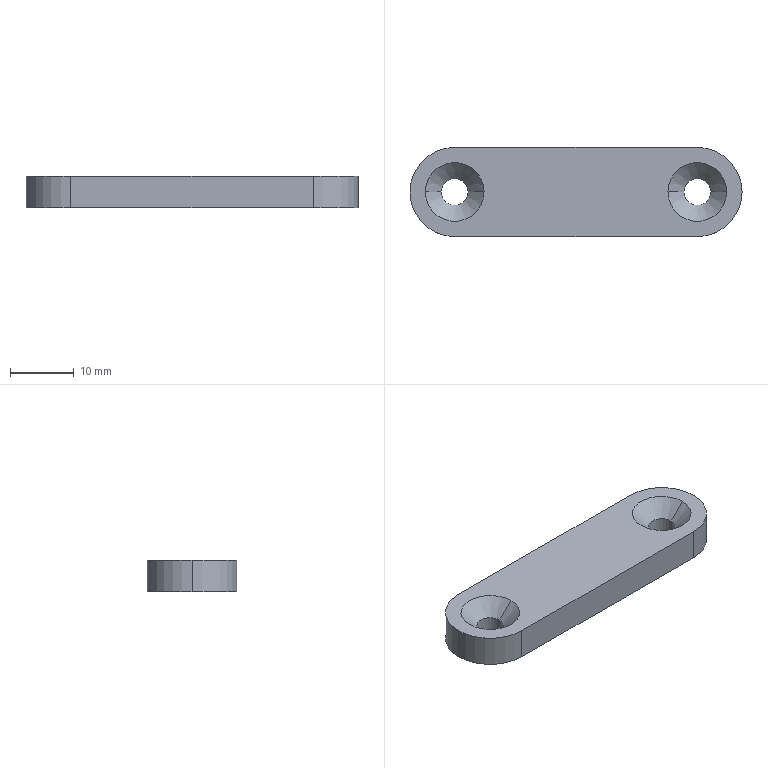Part | STEP file | Ngam kep 4 | 1 solid | 16 faces | box 52 x 14 x 5 mm | volume 3176 mm3 | cylinder 8 | cone 4 | plane 4 | commonest cylinder face diameters 4.2 x4 14 x4
STEP:
#1=CARTESIAN_POINT('',(0.,0.,0.));
#2=DIRECTION('',(0.,0.,1.));
#3=DIRECTION('',(1.,0.,0.));
#4=AXIS2_PLACEMENT_3D('',#1,#2,#3);
#5=CARTESIAN_POINT('',(-16.9,0.,2.5));
#6=VERTEX_POINT('',#5);
#7=CARTESIAN_POINT('',(-14.4,0.,5.));
#8=VERTEX_POINT('',#7);
#9=CARTESIAN_POINT('',(-16.9,0.,2.5));
#10=DIRECTION('',(0.7071,0.,0.7071));
#11=VECTOR('',#10,1.);
#12=LINE('',#9,#11);
#13=CARTESIAN_POINT('',(-19.,0.,2.5));
#14=DIRECTION('',(0.,0.,1.));
#15=DIRECTION('',(1.,0.,0.));
#16=AXIS2_PLACEMENT_3D('',#13,#14,#15);
#17=CONICAL_SURFACE('',#16,2.1,0.7854);
#18=CARTESIAN_POINT('',(6.283,0.));
#19=DIRECTION('',(0.,1.));
#20=VECTOR('',#19,1.);
#21=LINE('',#18,#20);
#22=(GEOMETRIC_REPRESENTATION_CONTEXT(2)PARAMETRIC_REPRESENTATION_CONTEXT()REPRESENTATION_CONTEXT('',''));
#23=DEFINITIONAL_REPRESENTATION('',(#21),#22);
#24=PCURVE('',#17,#23);
#25=CARTESIAN_POINT('',(-19.,0.,2.5));
#26=DIRECTION('',(0.,0.,1.));
#27=DIRECTION('',(1.,0.,0.));
#28=AXIS2_PLACEMENT_3D('',#25,#26,#27);
#29=CONICAL_SURFACE('',#28,2.1,0.7854);
#30=CARTESIAN_POINT('',(0.,0.));
#31=DIRECTION('',(0.,1.));
#32=VECTOR('',#31,1.);
#33=LINE('',#30,#32);
#34=(GEOMETRIC_REPRESENTATION_CONTEXT(2)PARAMETRIC_REPRESENTATION_CONTEXT()REPRESENTATION_CONTEXT('',''));
#35=DEFINITIONAL_REPRESENTATION('',(#33),#34);
#36=PCURVE('',#29,#35);
#37=SURFACE_CURVE('',#12,(#24,#36),.PCURVE_S1.);
#38=EDGE_CURVE('',#6,#8,#37,.T.);
#39=ORIENTED_EDGE('',*,*,#38,.T.);
#40=CARTESIAN_POINT('',(-23.6,0.,5.));
#41=VERTEX_POINT('',#40);
#42=CARTESIAN_POINT('',(-19.,0.,5.));
#43=DIRECTION('',(0.,0.,-1.));
#44=DIRECTION('',(-1.,0.,0.));
#45=AXIS2_PLACEMENT_3D('',#42,#43,#44);
#46=CIRCLE('',#45,4.6);
#47=CARTESIAN_POINT('',(9.425,2.5));
#48=DIRECTION('',(-1.,0.));
#49=VECTOR('',#48,1.);
#50=LINE('',#47,#49);
#51=(GEOMETRIC_REPRESENTATION_CONTEXT(2)PARAMETRIC_REPRESENTATION_CONTEXT()REPRESENTATION_CONTEXT('',''));
#52=DEFINITIONAL_REPRESENTATION('',(#50),#51);
#53=PCURVE('',#17,#52);
#54=CARTESIAN_POINT('',(0.,0.,5.));
#55=DIRECTION('',(0.,0.,-1.));
#56=DIRECTION('',(-1.,0.,0.));
#57=AXIS2_PLACEMENT_3D('',#54,#55,#56);
#58=PLANE('',#57);
#59=CARTESIAN_POINT('',(19.,0.));
#60=DIRECTION('',(1.,0.));
#61=AXIS2_PLACEMENT_2D('',#59,#60);
#62=CIRCLE('',#61,4.6);
#63=(GEOMETRIC_REPRESENTATION_CONTEXT(2)PARAMETRIC_REPRESENTATION_CONTEXT()REPRESENTATION_CONTEXT('',''));
#64=DEFINITIONAL_REPRESENTATION('',(#62),#63);
#65=PCURVE('',#58,#64);
#66=SURFACE_CURVE('',#46,(#53,#65),.PCURVE_S1.);
#67=EDGE_CURVE('',#8,#41,#66,.T.);
#68=ORIENTED_EDGE('',*,*,#67,.T.);
#69=CARTESIAN_POINT('',(-21.1,0.,2.5));
#70=VERTEX_POINT('',#69);
#71=CARTESIAN_POINT('',(-21.1,0.,2.5));
#72=DIRECTION('',(-0.7071,0.,0.7071));
#73=VECTOR('',#72,1.);
#74=LINE('',#71,#73);
#75=CARTESIAN_POINT('',(3.142,0.));
#76=DIRECTION('',(0.,1.));
#77=VECTOR('',#76,1.);
#78=LINE('',#75,#77);
#79=(GEOMETRIC_REPRESENTATION_CONTEXT(2)PARAMETRIC_REPRESENTATION_CONTEXT()REPRESENTATION_CONTEXT('',''));
#80=DEFINITIONAL_REPRESENTATION('',(#78),#79);
#81=PCURVE('',#17,#80);
#82=CARTESIAN_POINT('',(3.142,0.));
#83=DIRECTION('',(0.,1.));
#84=VECTOR('',#83,1.);
#85=LINE('',#82,#84);
#86=(GEOMETRIC_REPRESENTATION_CONTEXT(2)PARAMETRIC_REPRESENTATION_CONTEXT()REPRESENTATION_CONTEXT('',''));
#87=DEFINITIONAL_REPRESENTATION('',(#85),#86);
#88=PCURVE('',#29,#87);
#89=SURFACE_CURVE('',#74,(#81,#88),.PCURVE_S1.);
#90=EDGE_CURVE('',#70,#41,#89,.T.);
#91=ORIENTED_EDGE('',*,*,#90,.F.);
#92=CARTESIAN_POINT('',(-19.,0.,2.5));
#93=DIRECTION('',(0.,0.,1.));
#94=DIRECTION('',(-1.,0.,0.));
#95=AXIS2_PLACEMENT_3D('',#92,#93,#94);
#96=CIRCLE('',#95,2.1);
#97=CARTESIAN_POINT('',(3.142,0.));
#98=DIRECTION('',(1.,0.));
#99=VECTOR('',#98,1.);
#100=LINE('',#97,#99);
#101=(GEOMETRIC_REPRESENTATION_CONTEXT(2)PARAMETRIC_REPRESENTATION_CONTEXT()REPRESENTATION_CONTEXT('',''));
#102=DEFINITIONAL_REPRESENTATION('',(#100),#101);
#103=PCURVE('',#17,#102);
#104=CARTESIAN_POINT('',(-19.,0.,5.));
#105=DIRECTION('',(0.,0.,-1.));
#106=DIRECTION('',(-1.,0.,0.));
#107=AXIS2_PLACEMENT_3D('',#104,#105,#106);
#108=CYLINDRICAL_SURFACE('',#107,2.1);
#109=CARTESIAN_POINT('',(6.283,2.5));
#110=DIRECTION('',(-1.,0.));
#111=VECTOR('',#110,1.);
#112=LINE('',#109,#111);
#113=(GEOMETRIC_REPRESENTATION_CONTEXT(2)PARAMETRIC_REPRESENTATION_CONTEXT()REPRESENTATION_CONTEXT('',''));
#114=DEFINITIONAL_REPRESENTATION('',(#112),#113);
#115=PCURVE('',#108,#114);
#116=SURFACE_CURVE('',#96,(#103,#115),.PCURVE_S1.);
#117=EDGE_CURVE('',#70,#6,#116,.T.);
#118=ORIENTED_EDGE('',*,*,#117,.T.);
#119=EDGE_LOOP('',(#39,#68,#91,#118));
#120=FACE_BOUND('',#119,.F.);
#121=ADVANCED_FACE('',(#120),#17,.F.);
#122=CARTESIAN_POINT('',(21.1,0.,2.5));
#123=VERTEX_POINT('',#122);
#124=CARTESIAN_POINT('',(23.6,0.,5.));
#125=VERTEX_POINT('',#124);
#126=CARTESIAN_POINT('',(21.1,0.,2.5));
#127=DIRECTION('',(0.7071,0.,0.7071));
#128=VECTOR('',#127,1.);
#129=LINE('',#126,#128);
#130=CARTESIAN_POINT('',(19.,0.,2.5));
#131=DIRECTION('',(0.,0.,1.));
#132=DIRECTION('',(1.,0.,0.));
#133=AXIS2_PLACEMENT_3D('',#130,#131,#132);
#134=CONICAL_SURFACE('',#133,2.1,0.7854);
#135=CARTESIAN_POINT('',(6.283,0.));
#136=DIRECTION('',(0.,1.));
#137=VECTOR('',#136,1.);
#138=LINE('',#135,#137);
#139=(GEOMETRIC_REPRESENTATION_CONTEXT(2)PARAMETRIC_REPRESENTATION_CONTEXT()REPRESENTATION_CONTEXT('',''));
#140=DEFINITIONAL_REPRESENTATION('',(#138),#139);
#141=PCURVE('',#134,#140);
#142=CARTESIAN_POINT('',(19.,0.,2.5));
#143=DIRECTION('',(0.,0.,1.));
#144=DIRECTION('',(1.,0.,0.));
#145=AXIS2_PLACEMENT_3D('',#142,#143,#144);
#146=CONICAL_SURFACE('',#145,2.1,0.7854);
#147=CARTESIAN_POINT('',(0.,0.));
#148=DIRECTION('',(0.,1.));
#149=VECTOR('',#148,1.);
#150=LINE('',#147,#149);
#151=(GEOMETRIC_REPRESENTATION_CONTEXT(2)PARAMETRIC_REPRESENTATION_CONTEXT()REPRESENTATION_CONTEXT('',''));
#152=DEFINITIONAL_REPRESENTATION('',(#150),#151);
#153=PCURVE('',#146,#152);
#154=SURFACE_CURVE('',#129,(#141,#153),.PCURVE_S1.);
#155=EDGE_CURVE('',#123,#125,#154,.T.);
#156=ORIENTED_EDGE('',*,*,#155,.T.);
#157=CARTESIAN_POINT('',(14.4,0.,5.));
#158=VERTEX_POINT('',#157);
#159=CARTESIAN_POINT('',(19.,0.,5.));
#160=DIRECTION('',(0.,0.,-1.));
#161=DIRECTION('',(-1.,0.,0.));
#162=AXIS2_PLACEMENT_3D('',#159,#160,#161);
#163=CIRCLE('',#162,4.6);
#164=CARTESIAN_POINT('',(9.425,2.5));
#165=DIRECTION('',(-1.,0.));
#166=VECTOR('',#165,1.);
#167=LINE('',#164,#166);
#168=(GEOMETRIC_REPRESENTATION_CONTEXT(2)PARAMETRIC_REPRESENTATION_CONTEXT()REPRESENTATION_CONTEXT('',''));
#169=DEFINITIONAL_REPRESENTATION('',(#167),#168);
#170=PCURVE('',#134,#169);
#171=CARTESIAN_POINT('',(-19.,0.));
#172=DIRECTION('',(1.,0.));
#173=AXIS2_PLACEMENT_2D('',#171,#172);
#174=CIRCLE('',#173,4.6);
#175=(GEOMETRIC_REPRESENTATION_CONTEXT(2)PARAMETRIC_REPRESENTATION_CONTEXT()REPRESENTATION_CONTEXT('',''));
#176=DEFINITIONAL_REPRESENTATION('',(#174),#175);
#177=PCURVE('',#58,#176);
#178=SURFACE_CURVE('',#163,(#170,#177),.PCURVE_S1.);
#179=EDGE_CURVE('',#125,#158,#178,.T.);
#180=ORIENTED_EDGE('',*,*,#179,.T.);
#181=CARTESIAN_POINT('',(16.9,0.,2.5));
#182=VERTEX_POINT('',#181);
#183=CARTESIAN_POINT('',(16.9,0.,2.5));
#184=DIRECTION('',(-0.7071,0.,0.7071));
#185=VECTOR('',#184,1.);
#186=LINE('',#183,#185);
#187=CARTESIAN_POINT('',(3.142,0.));
#188=DIRECTION('',(0.,1.));
#189=VECTOR('',#188,1.);
#190=LINE('',#187,#189);
#191=(GEOMETRIC_REPRESENTATION_CONTEXT(2)PARAMETRIC_REPRESENTATION_CONTEXT()REPRESENTATION_CONTEXT('',''));
#192=DEFINITIONAL_REPRESENTATION('',(#190),#191);
#193=PCURVE('',#134,#192);
#194=CARTESIAN_POINT('',(3.142,0.));
#195=DIRECTION('',(0.,1.));
#196=VECTOR('',#195,1.);
#197=LINE('',#194,#196);
#198=(GEOMETRIC_REPRESENTATION_CONTEXT(2)PARAMETRIC_REPRESENTATION_CONTEXT()REPRESENTATION_CONTEXT('',''));
#199=DEFINITIONAL_REPRESENTATION('',(#197),#198);
#200=PCURVE('',#146,#199);
#201=SURFACE_CURVE('',#186,(#193,#200),.PCURVE_S1.);
#202=EDGE_CURVE('',#182,#158,#201,.T.);
#203=ORIENTED_EDGE('',*,*,#202,.F.);
#204=CARTESIAN_POINT('',(19.,0.,2.5));
#205=DIRECTION('',(0.,0.,1.));
#206=DIRECTION('',(-1.,0.,0.));
#207=AXIS2_PLACEMENT_3D('',#204,#205,#206);
#208=CIRCLE('',#207,2.1);
#209=CARTESIAN_POINT('',(3.142,0.));
#210=DIRECTION('',(1.,0.));
#211=VECTOR('',#210,1.);
#212=LINE('',#209,#211);
#213=(GEOMETRIC_REPRESENTATION_CONTEXT(2)PARAMETRIC_REPRESENTATION_CONTEXT()REPRESENTATION_CONTEXT('',''));
#214=DEFINITIONAL_REPRESENTATION('',(#212),#213);
#215=PCURVE('',#134,#214);
#216=CARTESIAN_POINT('',(19.,0.,5.));
#217=DIRECTION('',(0.,0.,-1.));
#218=DIRECTION('',(-1.,0.,0.));
#219=AXIS2_PLACEMENT_3D('',#216,#217,#218);
#220=CYLINDRICAL_SURFACE('',#219,2.1);
#221=CARTESIAN_POINT('',(6.283,2.5));
#222=DIRECTION('',(-1.,0.));
#223=VECTOR('',#222,1.);
#224=LINE('',#221,#223);
#225=(GEOMETRIC_REPRESENTATION_CONTEXT(2)PARAMETRIC_REPRESENTATION_CONTEXT()REPRESENTATION_CONTEXT('',''));
#226=DEFINITIONAL_REPRESENTATION('',(#224),#225);
#227=PCURVE('',#220,#226);
#228=SURFACE_CURVE('',#208,(#215,#227),.PCURVE_S1.);
#229=EDGE_CURVE('',#182,#123,#228,.T.);
#230=ORIENTED_EDGE('',*,*,#229,.T.);
#231=EDGE_LOOP('',(#156,#180,#203,#230));
#232=FACE_BOUND('',#231,.F.);
#233=ADVANCED_FACE('',(#232),#134,.F.);
#234=CARTESIAN_POINT('',(16.9,0.,0.));
#235=VERTEX_POINT('',#234);
#236=CARTESIAN_POINT('',(16.9,0.,5.));
#237=DIRECTION('',(0.,0.,-1.));
#238=VECTOR('',#237,1.);
#239=LINE('',#236,#238);
#240=CARTESIAN_POINT('',(6.283,0.));
#241=DIRECTION('',(0.,1.));
#242=VECTOR('',#241,1.);
#243=LINE('',#240,#242);
#244=(GEOMETRIC_REPRESENTATION_CONTEXT(2)PARAMETRIC_REPRESENTATION_CONTEXT()REPRESENTATION_CONTEXT('',''));
#245=DEFINITIONAL_REPRESENTATION('',(#243),#244);
#246=PCURVE('',#220,#245);
#247=CARTESIAN_POINT('',(19.,0.,5.));
#248=DIRECTION('',(0.,0.,-1.));
#249=DIRECTION('',(-1.,0.,0.));
#250=AXIS2_PLACEMENT_3D('',#247,#248,#249);
#251=CYLINDRICAL_SURFACE('',#250,2.1);
#252=CARTESIAN_POINT('',(0.,0.));
#253=DIRECTION('',(0.,1.));
#254=VECTOR('',#253,1.);
#255=LINE('',#252,#254);
#256=(GEOMETRIC_REPRESENTATION_CONTEXT(2)PARAMETRIC_REPRESENTATION_CONTEXT()REPRESENTATION_CONTEXT('',''));
#257=DEFINITIONAL_REPRESENTATION('',(#255),#256);
#258=PCURVE('',#251,#257);
#259=SURFACE_CURVE('',#239,(#246,#258),.PCURVE_S1.);
#260=EDGE_CURVE('',#182,#235,#259,.T.);
#261=ORIENTED_EDGE('',*,*,#260,.T.);
#262=CARTESIAN_POINT('',(21.1,0.,0.));
#263=VERTEX_POINT('',#262);
#264=CARTESIAN_POINT('',(19.,0.,0.));
#265=DIRECTION('',(0.,0.,1.));
#266=DIRECTION('',(1.,0.,0.));
#267=AXIS2_PLACEMENT_3D('',#264,#265,#266);
#268=CIRCLE('',#267,2.1);
#269=CARTESIAN_POINT('',(9.425,5.));
#270=DIRECTION('',(-1.,0.));
#271=VECTOR('',#270,1.);
#272=LINE('',#269,#271);
#273=(GEOMETRIC_REPRESENTATION_CONTEXT(2)PARAMETRIC_REPRESENTATION_CONTEXT()REPRESENTATION_CONTEXT('',''));
#274=DEFINITIONAL_REPRESENTATION('',(#272),#273);
#275=PCURVE('',#220,#274);
#276=CARTESIAN_POINT('',(0.,0.,0.));
#277=DIRECTION('',(0.,0.,-1.));
#278=DIRECTION('',(-1.,0.,0.));
#279=AXIS2_PLACEMENT_3D('',#276,#277,#278);
#280=PLANE('',#279);
#281=CARTESIAN_POINT('',(-21.1,0.));
#282=CARTESIAN_POINT('',(-21.1,3.637));
#283=CARTESIAN_POINT('',(-17.95,1.819));
#284=CARTESIAN_POINT('',(-14.8,0.));
#285=CARTESIAN_POINT('',(-17.95,-1.819));
#286=CARTESIAN_POINT('',(-21.1,-3.637));
#287=CARTESIAN_POINT('',(-21.1,0.));
#288=(BOUNDED_CURVE()B_SPLINE_CURVE(2,(#281,#282,#283,#284,#285,#286,#287),.UNSPECIFIED.,.T.,.F.)B_SPLINE_CURVE_WITH_KNOTS((1,2,2,2,2,1),(-2.094,0.,2.094,4.189,6.283,8.378),.UNSPECIFIED.)CURVE()GEOMETRIC_REPRESENTATION_ITEM()RATIONAL_B_SPLINE_CURVE((1.,0.5,1.,0.5,1.,0.5,1.))REPRESENTATION_ITEM(''));
#289=(GEOMETRIC_REPRESENTATION_CONTEXT(2)PARAMETRIC_REPRESENTATION_CONTEXT()REPRESENTATION_CONTEXT('',''));
#290=DEFINITIONAL_REPRESENTATION('',(#288),#289);
#291=PCURVE('',#280,#290);
#292=SURFACE_CURVE('',#268,(#275,#291),.PCURVE_S1.);
#293=EDGE_CURVE('',#235,#263,#292,.T.);
#294=ORIENTED_EDGE('',*,*,#293,.T.);
#295=CARTESIAN_POINT('',(21.1,0.,5.));
#296=DIRECTION('',(0.,0.,-1.));
#297=VECTOR('',#296,1.);
#298=LINE('',#295,#297);
#299=CARTESIAN_POINT('',(3.142,0.));
#300=DIRECTION('',(0.,1.));
#301=VECTOR('',#300,1.);
#302=LINE('',#299,#301);
#303=(GEOMETRIC_REPRESENTATION_CONTEXT(2)PARAMETRIC_REPRESENTATION_CONTEXT()REPRESENTATION_CONTEXT('',''));
#304=DEFINITIONAL_REPRESENTATION('',(#302),#303);
#305=PCURVE('',#220,#304);
#306=CARTESIAN_POINT('',(3.142,0.));
#307=DIRECTION('',(0.,1.));
#308=VECTOR('',#307,1.);
#309=LINE('',#306,#308);
#310=(GEOMETRIC_REPRESENTATION_CONTEXT(2)PARAMETRIC_REPRESENTATION_CONTEXT()REPRESENTATION_CONTEXT('',''));
#311=DEFINITIONAL_REPRESENTATION('',(#309),#310);
#312=PCURVE('',#251,#311);
#313=SURFACE_CURVE('',#298,(#305,#312),.PCURVE_S1.);
#314=EDGE_CURVE('',#123,#263,#313,.T.);
#315=ORIENTED_EDGE('',*,*,#314,.F.);
#316=ORIENTED_EDGE('',*,*,#229,.F.);
#317=EDGE_LOOP('',(#261,#294,#315,#316));
#318=FACE_BOUND('',#317,.F.);
#319=ADVANCED_FACE('',(#318),#220,.F.);
#320=CARTESIAN_POINT('',(-21.1,0.,0.));
#321=VERTEX_POINT('',#320);
#322=CARTESIAN_POINT('',(-21.1,0.,5.));
#323=DIRECTION('',(0.,0.,-1.));
#324=VECTOR('',#323,1.);
#325=LINE('',#322,#324);
#326=CARTESIAN_POINT('',(6.283,0.));
#327=DIRECTION('',(0.,1.));
#328=VECTOR('',#327,1.);
#329=LINE('',#326,#328);
#330=(GEOMETRIC_REPRESENTATION_CONTEXT(2)PARAMETRIC_REPRESENTATION_CONTEXT()REPRESENTATION_CONTEXT('',''));
#331=DEFINITIONAL_REPRESENTATION('',(#329),#330);
#332=PCURVE('',#108,#331);
#333=CARTESIAN_POINT('',(-19.,0.,5.));
#334=DIRECTION('',(0.,0.,-1.));
#335=DIRECTION('',(-1.,0.,0.));
#336=AXIS2_PLACEMENT_3D('',#333,#334,#335);
#337=CYLINDRICAL_SURFACE('',#336,2.1);
#338=CARTESIAN_POINT('',(0.,0.));
#339=DIRECTION('',(0.,1.));
#340=VECTOR('',#339,1.);
#341=LINE('',#338,#340);
#342=(GEOMETRIC_REPRESENTATION_CONTEXT(2)PARAMETRIC_REPRESENTATION_CONTEXT()REPRESENTATION_CONTEXT('',''));
#343=DEFINITIONAL_REPRESENTATION('',(#341),#342);
#344=PCURVE('',#337,#343);
#345=SURFACE_CURVE('',#325,(#332,#344),.PCURVE_S1.);
#346=EDGE_CURVE('',#70,#321,#345,.T.);
#347=ORIENTED_EDGE('',*,*,#346,.T.);
#348=CARTESIAN_POINT('',(-16.9,0.,0.));
#349=VERTEX_POINT('',#348);
#350=CARTESIAN_POINT('',(-19.,0.,0.));
#351=DIRECTION('',(0.,0.,1.));
#352=DIRECTION('',(1.,0.,0.));
#353=AXIS2_PLACEMENT_3D('',#350,#351,#352);
#354=CIRCLE('',#353,2.1);
#355=CARTESIAN_POINT('',(9.425,5.));
#356=DIRECTION('',(-1.,0.));
#357=VECTOR('',#356,1.);
#358=LINE('',#355,#357);
#359=(GEOMETRIC_REPRESENTATION_CONTEXT(2)PARAMETRIC_REPRESENTATION_CONTEXT()REPRESENTATION_CONTEXT('',''));
#360=DEFINITIONAL_REPRESENTATION('',(#358),#359);
#361=PCURVE('',#108,#360);
#362=CARTESIAN_POINT('',(16.9,0.));
#363=CARTESIAN_POINT('',(16.9,3.637));
#364=CARTESIAN_POINT('',(20.05,1.819));
#365=CARTESIAN_POINT('',(23.2,0.));
#366=CARTESIAN_POINT('',(20.05,-1.819));
#367=CARTESIAN_POINT('',(16.9,-3.637));
#368=CARTESIAN_POINT('',(16.9,0.));
#369=(BOUNDED_CURVE()B_SPLINE_CURVE(2,(#362,#363,#364,#365,#366,#367,#368),.UNSPECIFIED.,.T.,.F.)B_SPLINE_CURVE_WITH_KNOTS((1,2,2,2,2,1),(-2.094,0.,2.094,4.189,6.283,8.378),.UNSPECIFIED.)CURVE()GEOMETRIC_REPRESENTATION_ITEM()RATIONAL_B_SPLINE_CURVE((1.,0.5,1.,0.5,1.,0.5,1.))REPRESENTATION_ITEM(''));
#370=(GEOMETRIC_REPRESENTATION_CONTEXT(2)PARAMETRIC_REPRESENTATION_CONTEXT()REPRESENTATION_CONTEXT('',''));
#371=DEFINITIONAL_REPRESENTATION('',(#369),#370);
#372=PCURVE('',#280,#371);
#373=SURFACE_CURVE('',#354,(#361,#372),.PCURVE_S1.);
#374=EDGE_CURVE('',#321,#349,#373,.T.);
#375=ORIENTED_EDGE('',*,*,#374,.T.);
#376=CARTESIAN_POINT('',(-16.9,0.,5.));
#377=DIRECTION('',(0.,0.,-1.));
#378=VECTOR('',#377,1.);
#379=LINE('',#376,#378);
#380=CARTESIAN_POINT('',(3.142,0.));
#381=DIRECTION('',(0.,1.));
#382=VECTOR('',#381,1.);
#383=LINE('',#380,#382);
#384=(GEOMETRIC_REPRESENTATION_CONTEXT(2)PARAMETRIC_REPRESENTATION_CONTEXT()REPRESENTATION_CONTEXT('',''));
#385=DEFINITIONAL_REPRESENTATION('',(#383),#384);
#386=PCURVE('',#108,#385);
#387=CARTESIAN_POINT('',(3.142,0.));
#388=DIRECTION('',(0.,1.));
#389=VECTOR('',#388,1.);
#390=LINE('',#387,#389);
#391=(GEOMETRIC_REPRESENTATION_CONTEXT(2)PARAMETRIC_REPRESENTATION_CONTEXT()REPRESENTATION_CONTEXT('',''));
#392=DEFINITIONAL_REPRESENTATION('',(#390),#391);
#393=PCURVE('',#337,#392);
#394=SURFACE_CURVE('',#379,(#386,#393),.PCURVE_S1.);
#395=EDGE_CURVE('',#6,#349,#394,.T.);
#396=ORIENTED_EDGE('',*,*,#395,.F.);
#397=ORIENTED_EDGE('',*,*,#117,.F.);
#398=EDGE_LOOP('',(#347,#375,#396,#397));
#399=FACE_BOUND('',#398,.F.);
#400=ADVANCED_FACE('',(#399),#108,.F.);
#401=ORIENTED_EDGE('',*,*,#179,.T.);
#402=CARTESIAN_POINT('',(19.,0.,5.));
#403=DIRECTION('',(0.,0.,-1.));
#404=DIRECTION('',(-1.,0.,0.));
#405=AXIS2_PLACEMENT_3D('',#402,#403,#404);
#406=CIRCLE('',#405,4.6);
#407=CARTESIAN_POINT('',(-19.,0.));
#408=DIRECTION('',(1.,0.));
#409=AXIS2_PLACEMENT_2D('',#407,#408);
#410=CIRCLE('',#409,4.6);
#411=(GEOMETRIC_REPRESENTATION_CONTEXT(2)PARAMETRIC_REPRESENTATION_CONTEXT()REPRESENTATION_CONTEXT('',''));
#412=DEFINITIONAL_REPRESENTATION('',(#410),#411);
#413=PCURVE('',#58,#412);
#414=CARTESIAN_POINT('',(3.142,2.5));
#415=DIRECTION('',(-1.,0.));
#416=VECTOR('',#415,1.);
#417=LINE('',#414,#416);
#418=(GEOMETRIC_REPRESENTATION_CONTEXT(2)PARAMETRIC_REPRESENTATION_CONTEXT()REPRESENTATION_CONTEXT('',''));
#419=DEFINITIONAL_REPRESENTATION('',(#417),#418);
#420=PCURVE('',#146,#419);
#421=SURFACE_CURVE('',#406,(#413,#420),.PCURVE_S1.);
#422=EDGE_CURVE('',#158,#125,#421,.T.);
#423=ORIENTED_EDGE('',*,*,#422,.T.);
#424=EDGE_LOOP('',(#401,#423));
#425=FACE_BOUND('',#424,.T.);
#426=ORIENTED_EDGE('',*,*,#67,.T.);
#427=CARTESIAN_POINT('',(-19.,0.,5.));
#428=DIRECTION('',(0.,0.,-1.));
#429=DIRECTION('',(-1.,0.,0.));
#430=AXIS2_PLACEMENT_3D('',#427,#428,#429);
#431=CIRCLE('',#430,4.6);
#432=CARTESIAN_POINT('',(19.,0.));
#433=DIRECTION('',(1.,0.));
#434=AXIS2_PLACEMENT_2D('',#432,#433);
#435=CIRCLE('',#434,4.6);
#436=(GEOMETRIC_REPRESENTATION_CONTEXT(2)PARAMETRIC_REPRESENTATION_CONTEXT()REPRESENTATION_CONTEXT('',''));
#437=DEFINITIONAL_REPRESENTATION('',(#435),#436);
#438=PCURVE('',#58,#437);
#439=CARTESIAN_POINT('',(3.142,2.5));
#440=DIRECTION('',(-1.,0.));
#441=VECTOR('',#440,1.);
#442=LINE('',#439,#441);
#443=(GEOMETRIC_REPRESENTATION_CONTEXT(2)PARAMETRIC_REPRESENTATION_CONTEXT()REPRESENTATION_CONTEXT('',''));
#444=DEFINITIONAL_REPRESENTATION('',(#442),#443);
#445=PCURVE('',#29,#444);
#446=SURFACE_CURVE('',#431,(#438,#445),.PCURVE_S1.);
#447=EDGE_CURVE('',#41,#8,#446,.T.);
#448=ORIENTED_EDGE('',*,*,#447,.T.);
#449=EDGE_LOOP('',(#426,#448));
#450=FACE_BOUND('',#449,.T.);
#451=CARTESIAN_POINT('',(-19.,7.,5.));
#452=VERTEX_POINT('',#451);
#453=CARTESIAN_POINT('',(-26.,0.,5.));
#454=VERTEX_POINT('',#453);
#455=CARTESIAN_POINT('',(-19.,0.,5.));
#456=DIRECTION('',(0.,0.,1.));
#457=DIRECTION('',(-1.,0.,0.));
#458=AXIS2_PLACEMENT_3D('',#455,#456,#457);
#459=CIRCLE('',#458,7.);
#460=CARTESIAN_POINT('',(26.,0.));
#461=CARTESIAN_POINT('',(26.,-12.124));
#462=CARTESIAN_POINT('',(15.5,-6.062));
#463=CARTESIAN_POINT('',(5.,0.));
#464=CARTESIAN_POINT('',(15.5,6.062));
#465=CARTESIAN_POINT('',(26.,12.124));
#466=CARTESIAN_POINT('',(26.,0.));
#467=(BOUNDED_CURVE()B_SPLINE_CURVE(2,(#460,#461,#462,#463,#464,#465,#466),.UNSPECIFIED.,.T.,.F.)B_SPLINE_CURVE_WITH_KNOTS((1,2,2,2,2,1),(-2.094,0.,2.094,4.189,6.283,8.378),.UNSPECIFIED.)CURVE()GEOMETRIC_REPRESENTATION_ITEM()RATIONAL_B_SPLINE_CURVE((1.,0.5,1.,0.5,1.,0.5,1.))REPRESENTATION_ITEM(''));
#468=(GEOMETRIC_REPRESENTATION_CONTEXT(2)PARAMETRIC_REPRESENTATION_CONTEXT()REPRESENTATION_CONTEXT('',''));
#469=DEFINITIONAL_REPRESENTATION('',(#467),#468);
#470=PCURVE('',#58,#469);
#471=CARTESIAN_POINT('',(-19.,0.,5.));
#472=DIRECTION('',(0.,0.,-1.));
#473=DIRECTION('',(-1.,0.,0.));
#474=AXIS2_PLACEMENT_3D('',#471,#472,#473);
#475=CYLINDRICAL_SURFACE('',#474,7.);
#476=CARTESIAN_POINT('',(6.283,0.));
#477=DIRECTION('',(-1.,0.));
#478=VECTOR('',#477,1.);
#479=LINE('',#476,#478);
#480=(GEOMETRIC_REPRESENTATION_CONTEXT(2)PARAMETRIC_REPRESENTATION_CONTEXT()REPRESENTATION_CONTEXT('',''));
#481=DEFINITIONAL_REPRESENTATION('',(#479),#480);
#482=PCURVE('',#475,#481);
#483=SURFACE_CURVE('',#459,(#470,#482),.PCURVE_S1.);
#484=EDGE_CURVE('',#452,#454,#483,.T.);
#485=ORIENTED_EDGE('',*,*,#484,.T.);
#486=CARTESIAN_POINT('',(-19.,-7.,5.));
#487=VERTEX_POINT('',#486);
#488=CARTESIAN_POINT('',(-19.,0.,5.));
#489=DIRECTION('',(0.,0.,1.));
#490=DIRECTION('',(-1.,0.,0.));
#491=AXIS2_PLACEMENT_3D('',#488,#489,#490);
#492=CIRCLE('',#491,7.);
#493=CARTESIAN_POINT('',(26.,0.));
#494=CARTESIAN_POINT('',(26.,-12.124));
#495=CARTESIAN_POINT('',(15.5,-6.062));
#496=CARTESIAN_POINT('',(5.,0.));
#497=CARTESIAN_POINT('',(15.5,6.062));
#498=CARTESIAN_POINT('',(26.,12.124));
#499=CARTESIAN_POINT('',(26.,0.));
#500=(BOUNDED_CURVE()B_SPLINE_CURVE(2,(#493,#494,#495,#496,#497,#498,#499),.UNSPECIFIED.,.T.,.F.)B_SPLINE_CURVE_WITH_KNOTS((1,2,2,2,2,1),(-2.094,0.,2.094,4.189,6.283,8.378),.UNSPECIFIED.)CURVE()GEOMETRIC_REPRESENTATION_ITEM()RATIONAL_B_SPLINE_CURVE((1.,0.5,1.,0.5,1.,0.5,1.))REPRESENTATION_ITEM(''));
#501=(GEOMETRIC_REPRESENTATION_CONTEXT(2)PARAMETRIC_REPRESENTATION_CONTEXT()REPRESENTATION_CONTEXT('',''));
#502=DEFINITIONAL_REPRESENTATION('',(#500),#501);
#503=PCURVE('',#58,#502);
#504=CARTESIAN_POINT('',(-19.,0.,5.));
#505=DIRECTION('',(0.,0.,-1.));
#506=DIRECTION('',(-1.,0.,0.));
#507=AXIS2_PLACEMENT_3D('',#504,#505,#506);
#508=CYLINDRICAL_SURFACE('',#507,7.);
#509=CARTESIAN_POINT('',(6.283,0.));
#510=DIRECTION('',(-1.,0.));
#511=VECTOR('',#510,1.);
#512=LINE('',#509,#511);
#513=(GEOMETRIC_REPRESENTATION_CONTEXT(2)PARAMETRIC_REPRESENTATION_CONTEXT()REPRESENTATION_CONTEXT('',''));
#514=DEFINITIONAL_REPRESENTATION('',(#512),#513);
#515=PCURVE('',#508,#514);
#516=SURFACE_CURVE('',#492,(#503,#515),.PCURVE_S1.);
#517=EDGE_CURVE('',#454,#487,#516,.T.);
#518=ORIENTED_EDGE('',*,*,#517,.T.);
#519=CARTESIAN_POINT('',(19.,-7.,5.));
#520=VERTEX_POINT('',#519);
#521=CARTESIAN_POINT('',(26.,-7.,5.));
#522=DIRECTION('',(1.,0.,0.));
#523=VECTOR('',#522,1.);
#524=LINE('',#521,#523);
#525=CARTESIAN_POINT('',(-26.,-7.));
#526=DIRECTION('',(-1.,0.));
#527=VECTOR('',#526,1.);
#528=LINE('',#525,#527);
#529=(GEOMETRIC_REPRESENTATION_CONTEXT(2)PARAMETRIC_REPRESENTATION_CONTEXT()REPRESENTATION_CONTEXT('',''));
#530=DEFINITIONAL_REPRESENTATION('',(#528),#529);
#531=PCURVE('',#58,#530);
#532=CARTESIAN_POINT('',(26.,-7.,5.));
#533=DIRECTION('',(0.,1.,0.));
#534=DIRECTION('',(-1.,0.,0.));
#535=AXIS2_PLACEMENT_3D('',#532,#533,#534);
#536=PLANE('',#535);
#537=CARTESIAN_POINT('',(0.,0.));
#538=DIRECTION('',(-1.,0.));
#539=VECTOR('',#538,1.);
#540=LINE('',#537,#539);
#541=(GEOMETRIC_REPRESENTATION_CONTEXT(2)PARAMETRIC_REPRESENTATION_CONTEXT()REPRESENTATION_CONTEXT('',''));
#542=DEFINITIONAL_REPRESENTATION('',(#540),#541);
#543=PCURVE('',#536,#542);
#544=SURFACE_CURVE('',#524,(#531,#543),.PCURVE_S1.);
#545=EDGE_CURVE('',#487,#520,#544,.T.);
#546=ORIENTED_EDGE('',*,*,#545,.T.);
#547=CARTESIAN_POINT('',(26.,0.,5.));
#548=VERTEX_POINT('',#547);
#549=CARTESIAN_POINT('',(19.,0.,5.));
#550=DIRECTION('',(0.,0.,1.));
#551=DIRECTION('',(-1.,0.,0.));
#552=AXIS2_PLACEMENT_3D('',#549,#550,#551);
#553=CIRCLE('',#552,7.);
#554=CARTESIAN_POINT('',(-12.,0.));
#555=CARTESIAN_POINT('',(-12.,-12.124));
#556=CARTESIAN_POINT('',(-22.5,-6.062));
#557=CARTESIAN_POINT('',(-33.,0.));
#558=CARTESIAN_POINT('',(-22.5,6.062));
#559=CARTESIAN_POINT('',(-12.,12.124));
#560=CARTESIAN_POINT('',(-12.,0.));
#561=(BOUNDED_CURVE()B_SPLINE_CURVE(2,(#554,#555,#556,#557,#558,#559,#560),.UNSPECIFIED.,.T.,.F.)B_SPLINE_CURVE_WITH_KNOTS((1,2,2,2,2,1),(-2.094,0.,2.094,4.189,6.283,8.378),.UNSPECIFIED.)CURVE()GEOMETRIC_REPRESENTATION_ITEM()RATIONAL_B_SPLINE_CURVE((1.,0.5,1.,0.5,1.,0.5,1.))REPRESENTATION_ITEM(''));
#562=(GEOMETRIC_REPRESENTATION_CONTEXT(2)PARAMETRIC_REPRESENTATION_CONTEXT()REPRESENTATION_CONTEXT('',''));
#563=DEFINITIONAL_REPRESENTATION('',(#561),#562);
#564=PCURVE('',#58,#563);
#565=CARTESIAN_POINT('',(19.,0.,5.));
#566=DIRECTION('',(0.,0.,-1.));
#567=DIRECTION('',(-1.,0.,0.));
#568=AXIS2_PLACEMENT_3D('',#565,#566,#567);
#569=CYLINDRICAL_SURFACE('',#568,7.);
#570=CARTESIAN_POINT('',(6.283,0.));
#571=DIRECTION('',(-1.,0.));
#572=VECTOR('',#571,1.);
#573=LINE('',#570,#572);
#574=(GEOMETRIC_REPRESENTATION_CONTEXT(2)PARAMETRIC_REPRESENTATION_CONTEXT()REPRESENTATION_CONTEXT('',''));
#575=DEFINITIONAL_REPRESENTATION('',(#573),#574);
#576=PCURVE('',#569,#575);
#577=SURFACE_CURVE('',#553,(#564,#576),.PCURVE_S1.);
#578=EDGE_CURVE('',#520,#548,#577,.T.);
#579=ORIENTED_EDGE('',*,*,#578,.T.);
#580=CARTESIAN_POINT('',(19.,7.,5.));
#581=VERTEX_POINT('',#580);
#582=CARTESIAN_POINT('',(19.,0.,5.));
#583=DIRECTION('',(0.,0.,1.));
#584=DIRECTION('',(-1.,0.,0.));
#585=AXIS2_PLACEMENT_3D('',#582,#583,#584);
#586=CIRCLE('',#585,7.);
#587=CARTESIAN_POINT('',(-12.,0.));
#588=CARTESIAN_POINT('',(-12.,-12.124));
#589=CARTESIAN_POINT('',(-22.5,-6.062));
#590=CARTESIAN_POINT('',(-33.,0.));
#591=CARTESIAN_POINT('',(-22.5,6.062));
#592=CARTESIAN_POINT('',(-12.,12.124));
#593=CARTESIAN_POINT('',(-12.,0.));
#594=(BOUNDED_CURVE()B_SPLINE_CURVE(2,(#587,#588,#589,#590,#591,#592,#593),.UNSPECIFIED.,.T.,.F.)B_SPLINE_CURVE_WITH_KNOTS((1,2,2,2,2,1),(-2.094,0.,2.094,4.189,6.283,8.378),.UNSPECIFIED.)CURVE()GEOMETRIC_REPRESENTATION_ITEM()RATIONAL_B_SPLINE_CURVE((1.,0.5,1.,0.5,1.,0.5,1.))REPRESENTATION_ITEM(''));
#595=(GEOMETRIC_REPRESENTATION_CONTEXT(2)PARAMETRIC_REPRESENTATION_CONTEXT()REPRESENTATION_CONTEXT('',''));
#596=DEFINITIONAL_REPRESENTATION('',(#594),#595);
#597=PCURVE('',#58,#596);
#598=CARTESIAN_POINT('',(19.,0.,5.));
#599=DIRECTION('',(0.,0.,-1.));
#600=DIRECTION('',(-1.,0.,0.));
#601=AXIS2_PLACEMENT_3D('',#598,#599,#600);
#602=CYLINDRICAL_SURFACE('',#601,7.);
#603=CARTESIAN_POINT('',(6.283,0.));
#604=DIRECTION('',(-1.,0.));
#605=VECTOR('',#604,1.);
#606=LINE('',#603,#605);
#607=(GEOMETRIC_REPRESENTATION_CONTEXT(2)PARAMETRIC_REPRESENTATION_CONTEXT()REPRESENTATION_CONTEXT('',''));
#608=DEFINITIONAL_REPRESENTATION('',(#606),#607);
#609=PCURVE('',#602,#608);
#610=SURFACE_CURVE('',#586,(#597,#609),.PCURVE_S1.);
#611=EDGE_CURVE('',#548,#581,#610,.T.);
#612=ORIENTED_EDGE('',*,*,#611,.T.);
#613=CARTESIAN_POINT('',(-26.,7.,5.));
#614=DIRECTION('',(-1.,0.,0.));
#615=VECTOR('',#614,1.);
#616=LINE('',#613,#615);
#617=CARTESIAN_POINT('',(26.,7.));
#618=DIRECTION('',(1.,0.));
#619=VECTOR('',#618,1.);
#620=LINE('',#617,#619);
#621=(GEOMETRIC_REPRESENTATION_CONTEXT(2)PARAMETRIC_REPRESENTATION_CONTEXT()REPRESENTATION_CONTEXT('',''));
#622=DEFINITIONAL_REPRESENTATION('',(#620),#621);
#623=PCURVE('',#58,#622);
#624=CARTESIAN_POINT('',(-26.,7.,5.));
#625=DIRECTION('',(0.,-1.,0.));
#626=DIRECTION('',(0.,0.,-1.));
#627=AXIS2_PLACEMENT_3D('',#624,#625,#626);
#628=PLANE('',#627);
#629=CARTESIAN_POINT('',(0.,0.));
#630=DIRECTION('',(0.,-1.));
#631=VECTOR('',#630,1.);
#632=LINE('',#629,#631);
#633=(GEOMETRIC_REPRESENTATION_CONTEXT(2)PARAMETRIC_REPRESENTATION_CONTEXT()REPRESENTATION_CONTEXT('',''));
#634=DEFINITIONAL_REPRESENTATION('',(#632),#633);
#635=PCURVE('',#628,#634);
#636=SURFACE_CURVE('',#616,(#623,#635),.PCURVE_S1.);
#637=EDGE_CURVE('',#581,#452,#636,.T.);
#638=ORIENTED_EDGE('',*,*,#637,.T.);
#639=EDGE_LOOP('',(#485,#518,#546,#579,#612,#638));
#640=FACE_BOUND('',#639,.T.);
#641=ADVANCED_FACE('',(#425,#450,#640),#58,.F.);
#642=ORIENTED_EDGE('',*,*,#374,.T.);
#643=CARTESIAN_POINT('',(-19.,0.,0.));
#644=DIRECTION('',(0.,0.,1.));
#645=DIRECTION('',(1.,0.,0.));
#646=AXIS2_PLACEMENT_3D('',#643,#644,#645);
#647=CIRCLE('',#646,2.1);
#648=CARTESIAN_POINT('',(16.9,0.));
#649=CARTESIAN_POINT('',(16.9,3.637));
#650=CARTESIAN_POINT('',(20.05,1.819));
#651=CARTESIAN_POINT('',(23.2,0.));
#652=CARTESIAN_POINT('',(20.05,-1.819));
#653=CARTESIAN_POINT('',(16.9,-3.637));
#654=CARTESIAN_POINT('',(16.9,0.));
#655=(BOUNDED_CURVE()B_SPLINE_CURVE(2,(#648,#649,#650,#651,#652,#653,#654),.UNSPECIFIED.,.T.,.F.)B_SPLINE_CURVE_WITH_KNOTS((1,2,2,2,2,1),(-2.094,0.,2.094,4.189,6.283,8.378),.UNSPECIFIED.)CURVE()GEOMETRIC_REPRESENTATION_ITEM()RATIONAL_B_SPLINE_CURVE((1.,0.5,1.,0.5,1.,0.5,1.))REPRESENTATION_ITEM(''));
#656=(GEOMETRIC_REPRESENTATION_CONTEXT(2)PARAMETRIC_REPRESENTATION_CONTEXT()REPRESENTATION_CONTEXT('',''));
#657=DEFINITIONAL_REPRESENTATION('',(#655),#656);
#658=PCURVE('',#280,#657);
#659=CARTESIAN_POINT('',(3.142,5.));
#660=DIRECTION('',(-1.,0.));
#661=VECTOR('',#660,1.);
#662=LINE('',#659,#661);
#663=(GEOMETRIC_REPRESENTATION_CONTEXT(2)PARAMETRIC_REPRESENTATION_CONTEXT()REPRESENTATION_CONTEXT('',''));
#664=DEFINITIONAL_REPRESENTATION('',(#662),#663);
#665=PCURVE('',#337,#664);
#666=SURFACE_CURVE('',#647,(#658,#665),.PCURVE_S1.);
#667=EDGE_CURVE('',#349,#321,#666,.T.);
#668=ORIENTED_EDGE('',*,*,#667,.T.);
#669=EDGE_LOOP('',(#642,#668));
#670=FACE_BOUND('',#669,.T.);
#671=CARTESIAN_POINT('',(-19.,-7.,0.));
#672=VERTEX_POINT('',#671);
#673=CARTESIAN_POINT('',(19.,-7.,0.));
#674=VERTEX_POINT('',#673);
#675=CARTESIAN_POINT('',(26.,-7.,0.));
#676=DIRECTION('',(1.,0.,0.));
#677=VECTOR('',#676,1.);
#678=LINE('',#675,#677);
#679=CARTESIAN_POINT('',(-26.,-7.));
#680=DIRECTION('',(-1.,0.));
#681=VECTOR('',#680,1.);
#682=LINE('',#679,#681);
#683=(GEOMETRIC_REPRESENTATION_CONTEXT(2)PARAMETRIC_REPRESENTATION_CONTEXT()REPRESENTATION_CONTEXT('',''));
#684=DEFINITIONAL_REPRESENTATION('',(#682),#683);
#685=PCURVE('',#280,#684);
#686=CARTESIAN_POINT('',(0.,-5.));
#687=DIRECTION('',(-1.,0.));
#688=VECTOR('',#687,1.);
#689=LINE('',#686,#688);
#690=(GEOMETRIC_REPRESENTATION_CONTEXT(2)PARAMETRIC_REPRESENTATION_CONTEXT()REPRESENTATION_CONTEXT('',''));
#691=DEFINITIONAL_REPRESENTATION('',(#689),#690);
#692=PCURVE('',#536,#691);
#693=SURFACE_CURVE('',#678,(#685,#692),.PCURVE_S1.);
#694=EDGE_CURVE('',#672,#674,#693,.T.);
#695=ORIENTED_EDGE('',*,*,#694,.F.);
#696=CARTESIAN_POINT('',(-26.,0.,0.));
#697=VERTEX_POINT('',#696);
#698=CARTESIAN_POINT('',(-19.,0.,0.));
#699=DIRECTION('',(0.,0.,-1.));
#700=DIRECTION('',(-1.,0.,0.));
#701=AXIS2_PLACEMENT_3D('',#698,#699,#700);
#702=CIRCLE('',#701,7.);
#703=CARTESIAN_POINT('',(19.,0.));
#704=DIRECTION('',(1.,0.));
#705=AXIS2_PLACEMENT_2D('',#703,#704);
#706=CIRCLE('',#705,7.);
#707=(GEOMETRIC_REPRESENTATION_CONTEXT(2)PARAMETRIC_REPRESENTATION_CONTEXT()REPRESENTATION_CONTEXT('',''));
#708=DEFINITIONAL_REPRESENTATION('',(#706),#707);
#709=PCURVE('',#280,#708);
#710=CARTESIAN_POINT('',(0.,5.));
#711=DIRECTION('',(1.,0.));
#712=VECTOR('',#711,1.);
#713=LINE('',#710,#712);
#714=(GEOMETRIC_REPRESENTATION_CONTEXT(2)PARAMETRIC_REPRESENTATION_CONTEXT()REPRESENTATION_CONTEXT('',''));
#715=DEFINITIONAL_REPRESENTATION('',(#713),#714);
#716=PCURVE('',#508,#715);
#717=SURFACE_CURVE('',#702,(#709,#716),.PCURVE_S1.);
#718=EDGE_CURVE('',#672,#697,#717,.T.);
#719=ORIENTED_EDGE('',*,*,#718,.T.);
#720=CARTESIAN_POINT('',(-19.,7.,0.));
#721=VERTEX_POINT('',#720);
#722=CARTESIAN_POINT('',(-19.,0.,0.));
#723=DIRECTION('',(0.,0.,-1.));
#724=DIRECTION('',(-1.,0.,0.));
#725=AXIS2_PLACEMENT_3D('',#722,#723,#724);
#726=CIRCLE('',#725,7.);
#727=CARTESIAN_POINT('',(19.,0.));
#728=DIRECTION('',(1.,0.));
#729=AXIS2_PLACEMENT_2D('',#727,#728);
#730=CIRCLE('',#729,7.);
#731=(GEOMETRIC_REPRESENTATION_CONTEXT(2)PARAMETRIC_REPRESENTATION_CONTEXT()REPRESENTATION_CONTEXT('',''));
#732=DEFINITIONAL_REPRESENTATION('',(#730),#731);
#733=PCURVE('',#280,#732);
#734=CARTESIAN_POINT('',(0.,5.));
#735=DIRECTION('',(1.,0.));
#736=VECTOR('',#735,1.);
#737=LINE('',#734,#736);
#738=(GEOMETRIC_REPRESENTATION_CONTEXT(2)PARAMETRIC_REPRESENTATION_CONTEXT()REPRESENTATION_CONTEXT('',''));
#739=DEFINITIONAL_REPRESENTATION('',(#737),#738);
#740=PCURVE('',#475,#739);
#741=SURFACE_CURVE('',#726,(#733,#740),.PCURVE_S1.);
#742=EDGE_CURVE('',#697,#721,#741,.T.);
#743=ORIENTED_EDGE('',*,*,#742,.T.);
#744=CARTESIAN_POINT('',(19.,7.,0.));
#745=VERTEX_POINT('',#744);
#746=CARTESIAN_POINT('',(-26.,7.,0.));
#747=DIRECTION('',(-1.,0.,0.));
#748=VECTOR('',#747,1.);
#749=LINE('',#746,#748);
#750=CARTESIAN_POINT('',(26.,7.));
#751=DIRECTION('',(1.,0.));
#752=VECTOR('',#751,1.);
#753=LINE('',#750,#752);
#754=(GEOMETRIC_REPRESENTATION_CONTEXT(2)PARAMETRIC_REPRESENTATION_CONTEXT()REPRESENTATION_CONTEXT('',''));
#755=DEFINITIONAL_REPRESENTATION('',(#753),#754);
#756=PCURVE('',#280,#755);
#757=CARTESIAN_POINT('',(5.,0.));
#758=DIRECTION('',(0.,-1.));
#759=VECTOR('',#758,1.);
#760=LINE('',#757,#759);
#761=(GEOMETRIC_REPRESENTATION_CONTEXT(2)PARAMETRIC_REPRESENTATION_CONTEXT()REPRESENTATION_CONTEXT('',''));
#762=DEFINITIONAL_REPRESENTATION('',(#760),#761);
#763=PCURVE('',#628,#762);
#764=SURFACE_CURVE('',#749,(#756,#763),.PCURVE_S1.);
#765=EDGE_CURVE('',#745,#721,#764,.T.);
#766=ORIENTED_EDGE('',*,*,#765,.F.);
#767=CARTESIAN_POINT('',(26.,0.,0.));
#768=VERTEX_POINT('',#767);
#769=CARTESIAN_POINT('',(19.,0.,0.));
#770=DIRECTION('',(0.,0.,-1.));
#771=DIRECTION('',(-1.,0.,0.));
#772=AXIS2_PLACEMENT_3D('',#769,#770,#771);
#773=CIRCLE('',#772,7.);
#774=CARTESIAN_POINT('',(-19.,0.));
#775=DIRECTION('',(1.,0.));
#776=AXIS2_PLACEMENT_2D('',#774,#775);
#777=CIRCLE('',#776,7.);
#778=(GEOMETRIC_REPRESENTATION_CONTEXT(2)PARAMETRIC_REPRESENTATION_CONTEXT()REPRESENTATION_CONTEXT('',''));
#779=DEFINITIONAL_REPRESENTATION('',(#777),#778);
#780=PCURVE('',#280,#779);
#781=CARTESIAN_POINT('',(0.,5.));
#782=DIRECTION('',(1.,0.));
#783=VECTOR('',#782,1.);
#784=LINE('',#781,#783);
#785=(GEOMETRIC_REPRESENTATION_CONTEXT(2)PARAMETRIC_REPRESENTATION_CONTEXT()REPRESENTATION_CONTEXT('',''));
#786=DEFINITIONAL_REPRESENTATION('',(#784),#785);
#787=PCURVE('',#602,#786);
#788=SURFACE_CURVE('',#773,(#780,#787),.PCURVE_S1.);
#789=EDGE_CURVE('',#745,#768,#788,.T.);
#790=ORIENTED_EDGE('',*,*,#789,.T.);
#791=CARTESIAN_POINT('',(19.,0.,0.));
#792=DIRECTION('',(0.,0.,-1.));
#793=DIRECTION('',(-1.,0.,0.));
#794=AXIS2_PLACEMENT_3D('',#791,#792,#793);
#795=CIRCLE('',#794,7.);
#796=CARTESIAN_POINT('',(-19.,0.));
#797=DIRECTION('',(1.,0.));
#798=AXIS2_PLACEMENT_2D('',#796,#797);
#799=CIRCLE('',#798,7.);
#800=(GEOMETRIC_REPRESENTATION_CONTEXT(2)PARAMETRIC_REPRESENTATION_CONTEXT()REPRESENTATION_CONTEXT('',''));
#801=DEFINITIONAL_REPRESENTATION('',(#799),#800);
#802=PCURVE('',#280,#801);
#803=CARTESIAN_POINT('',(0.,5.));
#804=DIRECTION('',(1.,0.));
#805=VECTOR('',#804,1.);
#806=LINE('',#803,#805);
#807=(GEOMETRIC_REPRESENTATION_CONTEXT(2)PARAMETRIC_REPRESENTATION_CONTEXT()REPRESENTATION_CONTEXT('',''));
#808=DEFINITIONAL_REPRESENTATION('',(#806),#807);
#809=PCURVE('',#569,#808);
#810=SURFACE_CURVE('',#795,(#802,#809),.PCURVE_S1.);
#811=EDGE_CURVE('',#768,#674,#810,.T.);
#812=ORIENTED_EDGE('',*,*,#811,.T.);
#813=EDGE_LOOP('',(#695,#719,#743,#766,#790,#812));
#814=FACE_BOUND('',#813,.T.);
#815=ORIENTED_EDGE('',*,*,#293,.T.);
#816=CARTESIAN_POINT('',(19.,0.,0.));
#817=DIRECTION('',(0.,0.,1.));
#818=DIRECTION('',(1.,0.,0.));
#819=AXIS2_PLACEMENT_3D('',#816,#817,#818);
#820=CIRCLE('',#819,2.1);
#821=CARTESIAN_POINT('',(-21.1,0.));
#822=CARTESIAN_POINT('',(-21.1,3.637));
#823=CARTESIAN_POINT('',(-17.95,1.819));
#824=CARTESIAN_POINT('',(-14.8,0.));
#825=CARTESIAN_POINT('',(-17.95,-1.819));
#826=CARTESIAN_POINT('',(-21.1,-3.637));
#827=CARTESIAN_POINT('',(-21.1,0.));
#828=(BOUNDED_CURVE()B_SPLINE_CURVE(2,(#821,#822,#823,#824,#825,#826,#827),.UNSPECIFIED.,.T.,.F.)B_SPLINE_CURVE_WITH_KNOTS((1,2,2,2,2,1),(-2.094,0.,2.094,4.189,6.283,8.378),.UNSPECIFIED.)CURVE()GEOMETRIC_REPRESENTATION_ITEM()RATIONAL_B_SPLINE_CURVE((1.,0.5,1.,0.5,1.,0.5,1.))REPRESENTATION_ITEM(''));
#829=(GEOMETRIC_REPRESENTATION_CONTEXT(2)PARAMETRIC_REPRESENTATION_CONTEXT()REPRESENTATION_CONTEXT('',''));
#830=DEFINITIONAL_REPRESENTATION('',(#828),#829);
#831=PCURVE('',#280,#830);
#832=CARTESIAN_POINT('',(3.142,5.));
#833=DIRECTION('',(-1.,0.));
#834=VECTOR('',#833,1.);
#835=LINE('',#832,#834);
#836=(GEOMETRIC_REPRESENTATION_CONTEXT(2)PARAMETRIC_REPRESENTATION_CONTEXT()REPRESENTATION_CONTEXT('',''));
#837=DEFINITIONAL_REPRESENTATION('',(#835),#836);
#838=PCURVE('',#251,#837);
#839=SURFACE_CURVE('',#820,(#831,#838),.PCURVE_S1.);
#840=EDGE_CURVE('',#263,#235,#839,.T.);
#841=ORIENTED_EDGE('',*,*,#840,.T.);
#842=EDGE_LOOP('',(#815,#841));
#843=FACE_BOUND('',#842,.T.);
#844=ADVANCED_FACE('',(#670,#814,#843),#280,.T.);
#845=ORIENTED_EDGE('',*,*,#545,.F.);
#846=CARTESIAN_POINT('',(-19.,-7.,5.));
#847=DIRECTION('',(0.,0.,-1.));
#848=VECTOR('',#847,1.);
#849=LINE('',#846,#848);
#850=CARTESIAN_POINT('',(45.,0.));
#851=DIRECTION('',(0.,-1.));
#852=VECTOR('',#851,1.);
#853=LINE('',#850,#852);
#854=(GEOMETRIC_REPRESENTATION_CONTEXT(2)PARAMETRIC_REPRESENTATION_CONTEXT()REPRESENTATION_CONTEXT('',''));
#855=DEFINITIONAL_REPRESENTATION('',(#853),#854);
#856=PCURVE('',#536,#855);
#857=CARTESIAN_POINT('',(4.712,0.));
#858=DIRECTION('',(0.,1.));
#859=VECTOR('',#858,1.);
#860=LINE('',#857,#859);
#861=(GEOMETRIC_REPRESENTATION_CONTEXT(2)PARAMETRIC_REPRESENTATION_CONTEXT()REPRESENTATION_CONTEXT('',''));
#862=DEFINITIONAL_REPRESENTATION('',(#860),#861);
#863=PCURVE('',#508,#862);
#864=SURFACE_CURVE('',#849,(#856,#863),.PCURVE_S1.);
#865=EDGE_CURVE('',#487,#672,#864,.T.);
#866=ORIENTED_EDGE('',*,*,#865,.T.);
#867=ORIENTED_EDGE('',*,*,#694,.T.);
#868=CARTESIAN_POINT('',(19.,-7.,5.));
#869=DIRECTION('',(0.,0.,1.));
#870=VECTOR('',#869,1.);
#871=LINE('',#868,#870);
#872=CARTESIAN_POINT('',(7.,0.));
#873=DIRECTION('',(0.,1.));
#874=VECTOR('',#873,1.);
#875=LINE('',#872,#874);
#876=(GEOMETRIC_REPRESENTATION_CONTEXT(2)PARAMETRIC_REPRESENTATION_CONTEXT()REPRESENTATION_CONTEXT('',''));
#877=DEFINITIONAL_REPRESENTATION('',(#875),#876);
#878=PCURVE('',#536,#877);
#879=CARTESIAN_POINT('',(4.712,0.));
#880=DIRECTION('',(0.,-1.));
#881=VECTOR('',#880,1.);
#882=LINE('',#879,#881);
#883=(GEOMETRIC_REPRESENTATION_CONTEXT(2)PARAMETRIC_REPRESENTATION_CONTEXT()REPRESENTATION_CONTEXT('',''));
#884=DEFINITIONAL_REPRESENTATION('',(#882),#883);
#885=PCURVE('',#569,#884);
#886=SURFACE_CURVE('',#871,(#878,#885),.PCURVE_S1.);
#887=EDGE_CURVE('',#674,#520,#886,.T.);
#888=ORIENTED_EDGE('',*,*,#887,.T.);
#889=EDGE_LOOP('',(#845,#866,#867,#888));
#890=FACE_BOUND('',#889,.T.);
#891=ADVANCED_FACE('',(#890),#536,.F.);
#892=ORIENTED_EDGE('',*,*,#765,.T.);
#893=CARTESIAN_POINT('',(-19.,7.,5.));
#894=DIRECTION('',(0.,0.,1.));
#895=VECTOR('',#894,1.);
#896=LINE('',#893,#895);
#897=CARTESIAN_POINT('',(0.,7.));
#898=DIRECTION('',(-1.,0.));
#899=VECTOR('',#898,1.);
#900=LINE('',#897,#899);
#901=(GEOMETRIC_REPRESENTATION_CONTEXT(2)PARAMETRIC_REPRESENTATION_CONTEXT()REPRESENTATION_CONTEXT('',''));
#902=DEFINITIONAL_REPRESENTATION('',(#900),#901);
#903=PCURVE('',#628,#902);
#904=CARTESIAN_POINT('',(1.571,0.));
#905=DIRECTION('',(0.,-1.));
#906=VECTOR('',#905,1.);
#907=LINE('',#904,#906);
#908=(GEOMETRIC_REPRESENTATION_CONTEXT(2)PARAMETRIC_REPRESENTATION_CONTEXT()REPRESENTATION_CONTEXT('',''));
#909=DEFINITIONAL_REPRESENTATION('',(#907),#908);
#910=PCURVE('',#475,#909);
#911=SURFACE_CURVE('',#896,(#903,#910),.PCURVE_S1.);
#912=EDGE_CURVE('',#721,#452,#911,.T.);
#913=ORIENTED_EDGE('',*,*,#912,.T.);
#914=ORIENTED_EDGE('',*,*,#637,.F.);
#915=CARTESIAN_POINT('',(19.,7.,5.));
#916=DIRECTION('',(0.,0.,-1.));
#917=VECTOR('',#916,1.);
#918=LINE('',#915,#917);
#919=CARTESIAN_POINT('',(0.,45.));
#920=DIRECTION('',(1.,0.));
#921=VECTOR('',#920,1.);
#922=LINE('',#919,#921);
#923=(GEOMETRIC_REPRESENTATION_CONTEXT(2)PARAMETRIC_REPRESENTATION_CONTEXT()REPRESENTATION_CONTEXT('',''));
#924=DEFINITIONAL_REPRESENTATION('',(#922),#923);
#925=PCURVE('',#628,#924);
#926=CARTESIAN_POINT('',(1.571,0.));
#927=DIRECTION('',(0.,1.));
#928=VECTOR('',#927,1.);
#929=LINE('',#926,#928);
#930=(GEOMETRIC_REPRESENTATION_CONTEXT(2)PARAMETRIC_REPRESENTATION_CONTEXT()REPRESENTATION_CONTEXT('',''));
#931=DEFINITIONAL_REPRESENTATION('',(#929),#930);
#932=PCURVE('',#602,#931);
#933=SURFACE_CURVE('',#918,(#925,#932),.PCURVE_S1.);
#934=EDGE_CURVE('',#581,#745,#933,.T.);
#935=ORIENTED_EDGE('',*,*,#934,.T.);
#936=EDGE_LOOP('',(#892,#913,#914,#935));
#937=FACE_BOUND('',#936,.T.);
#938=ADVANCED_FACE('',(#937),#628,.F.);
#939=ORIENTED_EDGE('',*,*,#667,.T.);
#940=ORIENTED_EDGE('',*,*,#346,.F.);
#941=CARTESIAN_POINT('',(-19.,0.,2.5));
#942=DIRECTION('',(0.,0.,1.));
#943=DIRECTION('',(-1.,0.,0.));
#944=AXIS2_PLACEMENT_3D('',#941,#942,#943);
#945=CIRCLE('',#944,2.1);
#946=CARTESIAN_POINT('',(6.283,2.5));
#947=DIRECTION('',(-1.,0.));
#948=VECTOR('',#947,1.);
#949=LINE('',#946,#948);
#950=(GEOMETRIC_REPRESENTATION_CONTEXT(2)PARAMETRIC_REPRESENTATION_CONTEXT()REPRESENTATION_CONTEXT('',''));
#951=DEFINITIONAL_REPRESENTATION('',(#949),#950);
#952=PCURVE('',#337,#951);
#953=CARTESIAN_POINT('',(-3.142,0.));
#954=DIRECTION('',(1.,0.));
#955=VECTOR('',#954,1.);
#956=LINE('',#953,#955);
#957=(GEOMETRIC_REPRESENTATION_CONTEXT(2)PARAMETRIC_REPRESENTATION_CONTEXT()REPRESENTATION_CONTEXT('',''));
#958=DEFINITIONAL_REPRESENTATION('',(#956),#957);
#959=PCURVE('',#29,#958);
#960=SURFACE_CURVE('',#945,(#952,#959),.PCURVE_S1.);
#961=EDGE_CURVE('',#6,#70,#960,.T.);
#962=ORIENTED_EDGE('',*,*,#961,.F.);
#963=ORIENTED_EDGE('',*,*,#395,.T.);
#964=EDGE_LOOP('',(#939,#940,#962,#963));
#965=FACE_BOUND('',#964,.F.);
#966=ADVANCED_FACE('',(#965),#337,.F.);
#967=ORIENTED_EDGE('',*,*,#840,.T.);
#968=ORIENTED_EDGE('',*,*,#260,.F.);
#969=CARTESIAN_POINT('',(19.,0.,2.5));
#970=DIRECTION('',(0.,0.,1.));
#971=DIRECTION('',(-1.,0.,0.));
#972=AXIS2_PLACEMENT_3D('',#969,#970,#971);
#973=CIRCLE('',#972,2.1);
#974=CARTESIAN_POINT('',(6.283,2.5));
#975=DIRECTION('',(-1.,0.));
#976=VECTOR('',#975,1.);
#977=LINE('',#974,#976);
#978=(GEOMETRIC_REPRESENTATION_CONTEXT(2)PARAMETRIC_REPRESENTATION_CONTEXT()REPRESENTATION_CONTEXT('',''));
#979=DEFINITIONAL_REPRESENTATION('',(#977),#978);
#980=PCURVE('',#251,#979);
#981=CARTESIAN_POINT('',(-3.142,0.));
#982=DIRECTION('',(1.,0.));
#983=VECTOR('',#982,1.);
#984=LINE('',#981,#983);
#985=(GEOMETRIC_REPRESENTATION_CONTEXT(2)PARAMETRIC_REPRESENTATION_CONTEXT()REPRESENTATION_CONTEXT('',''));
#986=DEFINITIONAL_REPRESENTATION('',(#984),#985);
#987=PCURVE('',#146,#986);
#988=SURFACE_CURVE('',#973,(#980,#987),.PCURVE_S1.);
#989=EDGE_CURVE('',#123,#182,#988,.T.);
#990=ORIENTED_EDGE('',*,*,#989,.F.);
#991=ORIENTED_EDGE('',*,*,#314,.T.);
#992=EDGE_LOOP('',(#967,#968,#990,#991));
#993=FACE_BOUND('',#992,.F.);
#994=ADVANCED_FACE('',(#993),#251,.F.);
#995=CARTESIAN_POINT('',(-26.,0.,5.));
#996=DIRECTION('',(0.,0.,-1.));
#997=VECTOR('',#996,1.);
#998=LINE('',#995,#997);
#999=CARTESIAN_POINT('',(0.,0.));
#1000=DIRECTION('',(0.,1.));
#1001=VECTOR('',#1000,1.);
#1002=LINE('',#999,#1001);
#1003=(GEOMETRIC_REPRESENTATION_CONTEXT(2)PARAMETRIC_REPRESENTATION_CONTEXT()REPRESENTATION_CONTEXT('',''));
#1004=DEFINITIONAL_REPRESENTATION('',(#1002),#1003);
#1005=PCURVE('',#475,#1004);
#1006=CARTESIAN_POINT('',(6.283,0.));
#1007=DIRECTION('',(0.,1.));
#1008=VECTOR('',#1007,1.);
#1009=LINE('',#1006,#1008);
#1010=(GEOMETRIC_REPRESENTATION_CONTEXT(2)PARAMETRIC_REPRESENTATION_CONTEXT()REPRESENTATION_CONTEXT('',''));
#1011=DEFINITIONAL_REPRESENTATION('',(#1009),#1010);
#1012=PCURVE('',#508,#1011);
#1013=SURFACE_CURVE('',#998,(#1005,#1012),.PCURVE_S1.);
#1014=EDGE_CURVE('',#454,#697,#1013,.T.);
#1015=ORIENTED_EDGE('',*,*,#1014,.F.);
#1016=ORIENTED_EDGE('',*,*,#484,.F.);
#1017=ORIENTED_EDGE('',*,*,#912,.F.);
#1018=ORIENTED_EDGE('',*,*,#742,.F.);
#1019=EDGE_LOOP('',(#1015,#1016,#1017,#1018));
#1020=FACE_BOUND('',#1019,.T.);
#1021=ADVANCED_FACE('',(#1020),#475,.T.);
#1022=ORIENTED_EDGE('',*,*,#517,.F.);
#1023=ORIENTED_EDGE('',*,*,#1014,.T.);
#1024=ORIENTED_EDGE('',*,*,#718,.F.);
#1025=ORIENTED_EDGE('',*,*,#865,.F.);
#1026=EDGE_LOOP('',(#1022,#1023,#1024,#1025));
#1027=FACE_BOUND('',#1026,.T.);
#1028=ADVANCED_FACE('',(#1027),#508,.T.);
#1029=ORIENTED_EDGE('',*,*,#934,.F.);
#1030=ORIENTED_EDGE('',*,*,#611,.F.);
#1031=CARTESIAN_POINT('',(26.,0.,5.));
#1032=DIRECTION('',(0.,0.,1.));
#1033=VECTOR('',#1032,1.);
#1034=LINE('',#1031,#1033);
#1035=CARTESIAN_POINT('',(3.142,0.));
#1036=DIRECTION('',(0.,-1.));
#1037=VECTOR('',#1036,1.);
#1038=LINE('',#1035,#1037);
#1039=(GEOMETRIC_REPRESENTATION_CONTEXT(2)PARAMETRIC_REPRESENTATION_CONTEXT()REPRESENTATION_CONTEXT('',''));
#1040=DEFINITIONAL_REPRESENTATION('',(#1038),#1039);
#1041=PCURVE('',#602,#1040);
#1042=CARTESIAN_POINT('',(3.142,0.));
#1043=DIRECTION('',(0.,-1.));
#1044=VECTOR('',#1043,1.);
#1045=LINE('',#1042,#1044);
#1046=(GEOMETRIC_REPRESENTATION_CONTEXT(2)PARAMETRIC_REPRESENTATION_CONTEXT()REPRESENTATION_CONTEXT('',''));
#1047=DEFINITIONAL_REPRESENTATION('',(#1045),#1046);
#1048=PCURVE('',#569,#1047);
#1049=SURFACE_CURVE('',#1034,(#1041,#1048),.PCURVE_S1.);
#1050=EDGE_CURVE('',#768,#548,#1049,.T.);
#1051=ORIENTED_EDGE('',*,*,#1050,.F.);
#1052=ORIENTED_EDGE('',*,*,#789,.F.);
#1053=EDGE_LOOP('',(#1029,#1030,#1051,#1052));
#1054=FACE_BOUND('',#1053,.T.);
#1055=ADVANCED_FACE('',(#1054),#602,.T.);
#1056=ORIENTED_EDGE('',*,*,#578,.F.);
#1057=ORIENTED_EDGE('',*,*,#887,.F.);
#1058=ORIENTED_EDGE('',*,*,#811,.F.);
#1059=ORIENTED_EDGE('',*,*,#1050,.T.);
#1060=EDGE_LOOP('',(#1056,#1057,#1058,#1059));
#1061=FACE_BOUND('',#1060,.T.);
#1062=ADVANCED_FACE('',(#1061),#569,.T.);
#1063=ORIENTED_EDGE('',*,*,#422,.T.);
#1064=ORIENTED_EDGE('',*,*,#155,.F.);
#1065=ORIENTED_EDGE('',*,*,#989,.T.);
#1066=ORIENTED_EDGE('',*,*,#202,.T.);
#1067=EDGE_LOOP('',(#1063,#1064,#1065,#1066));
#1068=FACE_BOUND('',#1067,.F.);
#1069=ADVANCED_FACE('',(#1068),#146,.F.);
#1070=ORIENTED_EDGE('',*,*,#447,.T.);
#1071=ORIENTED_EDGE('',*,*,#38,.F.);
#1072=ORIENTED_EDGE('',*,*,#961,.T.);
#1073=ORIENTED_EDGE('',*,*,#90,.T.);
#1074=EDGE_LOOP('',(#1070,#1071,#1072,#1073));
#1075=FACE_BOUND('',#1074,.F.);
#1076=ADVANCED_FACE('',(#1075),#29,.F.);
#1077=CLOSED_SHELL('',(#121,#233,#319,#400,#641,#844,#891,#938,#966,#994,#1021,#1028,#1055,#1062,#1069,#1076));
#1078=MANIFOLD_SOLID_BREP('',#1077);
#1079=(LENGTH_UNIT()NAMED_UNIT(*)SI_UNIT(.MILLI.,.METRE.));
#1080=UNCERTAINTY_MEASURE_WITH_UNIT(LENGTH_MEASURE(0.0000001),#1079,'','');
#1081=(NAMED_UNIT(*)PLANE_ANGLE_UNIT()SI_UNIT($,.RADIAN.));
#1082=(NAMED_UNIT(*)SI_UNIT($,.STERADIAN.)SOLID_ANGLE_UNIT());
#1083=(GEOMETRIC_REPRESENTATION_CONTEXT(3)GLOBAL_UNCERTAINTY_ASSIGNED_CONTEXT((#1080))GLOBAL_UNIT_ASSIGNED_CONTEXT((#1079,#1081,#1082))REPRESENTATION_CONTEXT('',''));
#1084=ADVANCED_BREP_SHAPE_REPRESENTATION('',(#4,#1078),#1083);